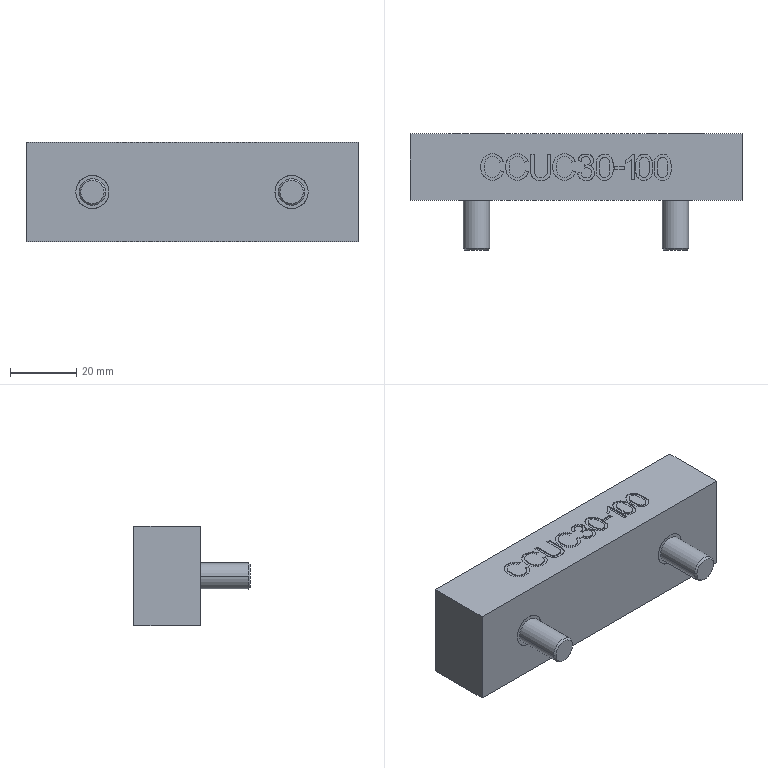Part | CATIA | 3 solids | 205 faces | box 100 x 35 x 30 mm | volume 56836 mm3 | plane 113 | cylinder 80 | cone 12 | commonest cylinder face diameters 10 x12 17 x8 8 x4 16 x4 3.298 x3 3.935 x3